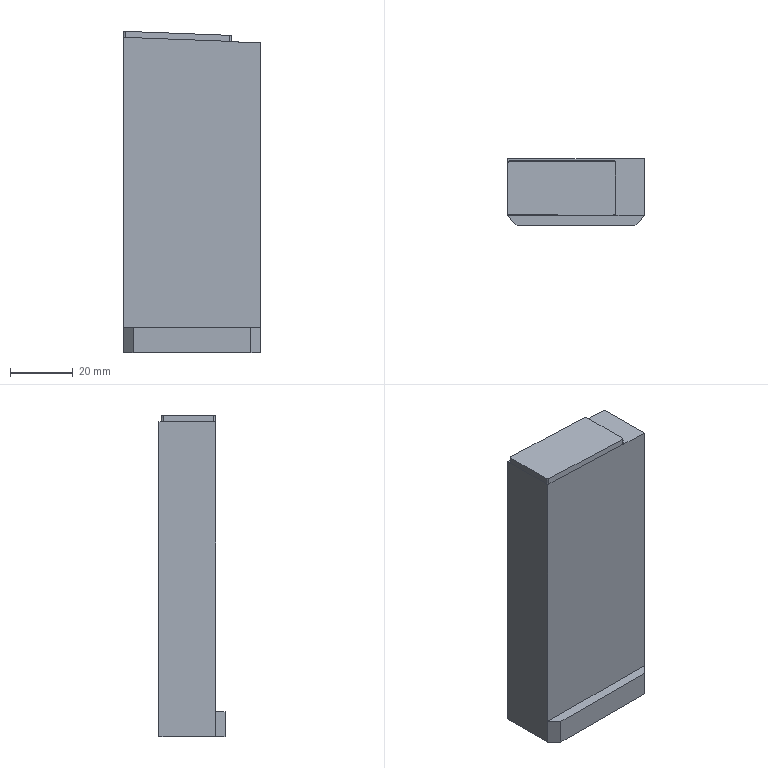Part | Creo | 1 solid | 134 faces | box 43.5 x 21 x 102.156 mm | volume 79919 mm3 | other 82 | plane 47 | spline 4 | cylinder 1 | commonest cylinder face diameters 2.697 x1